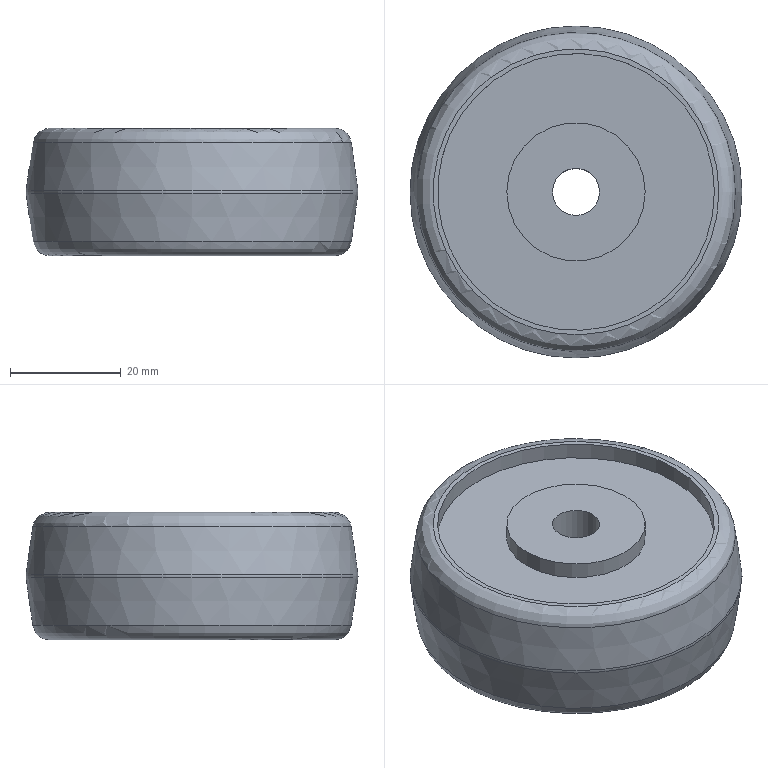Part | STEP file | Transport wheel | 1 solid | 16 faces | box 59.962 x 59.962 x 23 mm | volume 51034 mm3 | plane 6 | cylinder 5 | torus 3 | cone 2 | commonest cylinder face diameters 25 x2 50 x2 8.5 x1
STEP:
#1=CARTESIAN_POINT('',(0.,0.,0.));
#2=DIRECTION('',(0.,0.,1.));
#3=DIRECTION('',(1.,0.,0.));
#4=AXIS2_PLACEMENT_3D('',#1,#2,#3);
#5=CARTESIAN_POINT('',(-29.963,0.,11.772));
#6=VERTEX_POINT('',#5);
#7=CARTESIAN_POINT('',(29.963,0.,11.772));
#8=VERTEX_POINT('',#7);
#9=CARTESIAN_POINT('',(0.,0.,11.772));
#10=DIRECTION('',(0.,0.,1.));
#11=DIRECTION('',(1.,0.,0.));
#12=AXIS2_PLACEMENT_3D('',#9,#10,#11);
#13=CIRCLE('',#12,29.963);
#14=CARTESIAN_POINT('',(0.,0.,11.5));
#15=DIRECTION('',(0.,0.,-1.));
#16=DIRECTION('',(-1.,0.,0.));
#17=AXIS2_PLACEMENT_3D('',#14,#15,#16);
#18=TOROIDAL_SURFACE('',#17,27.981,2.);
#19=CARTESIAN_POINT('',(9.425,6.147));
#20=DIRECTION('',(-1.,0.));
#21=VECTOR('',#20,1.);
#22=LINE('',#19,#21);
#23=(GEOMETRIC_REPRESENTATION_CONTEXT(2)PARAMETRIC_REPRESENTATION_CONTEXT()REPRESENTATION_CONTEXT('',''));
#24=DEFINITIONAL_REPRESENTATION('',(#22),#23);
#25=PCURVE('',#18,#24);
#26=CARTESIAN_POINT('',(0.,0.,23.));
#27=DIRECTION('',(0.,0.,-1.));
#28=DIRECTION('',(-1.,0.,0.));
#29=AXIS2_PLACEMENT_3D('',#26,#27,#28);
#30=CONICAL_SURFACE('',#29,28.419,0.1366);
#31=CARTESIAN_POINT('',(9.425,11.228));
#32=DIRECTION('',(-1.,0.));
#33=VECTOR('',#32,1.);
#34=LINE('',#31,#33);
#35=(GEOMETRIC_REPRESENTATION_CONTEXT(2)PARAMETRIC_REPRESENTATION_CONTEXT()REPRESENTATION_CONTEXT('',''));
#36=DEFINITIONAL_REPRESENTATION('',(#34),#35);
#37=PCURVE('',#30,#36);
#38=SURFACE_CURVE('',#13,(#25,#37),.PCURVE_S1.);
#39=EDGE_CURVE('',#6,#8,#38,.T.);
#40=ORIENTED_EDGE('',*,*,#39,.F.);
#41=CARTESIAN_POINT('',(-29.963,0.,11.228));
#42=VERTEX_POINT('',#41);
#43=CARTESIAN_POINT('',(-29.963,0.,11.772));
#44=CARTESIAN_POINT('',(-29.981,0.,11.637));
#45=CARTESIAN_POINT('',(-29.987,0.,11.5));
#46=CARTESIAN_POINT('',(-29.981,0.,11.363));
#47=CARTESIAN_POINT('',(-29.963,0.,11.228));
#48=B_SPLINE_CURVE_WITH_KNOTS('',4,(#43,#44,#45,#46,#47),.UNSPECIFIED.,.F.,.F.,(5,5),(6.147,6.42),.PIECEWISE_BEZIER_KNOTS.);
#49=CARTESIAN_POINT('',(6.283,0.));
#50=DIRECTION('',(0.,1.));
#51=VECTOR('',#50,1.);
#52=LINE('',#49,#51);
#53=(GEOMETRIC_REPRESENTATION_CONTEXT(2)PARAMETRIC_REPRESENTATION_CONTEXT()REPRESENTATION_CONTEXT('',''));
#54=DEFINITIONAL_REPRESENTATION('',(#52),#53);
#55=PCURVE('',#18,#54);
#56=CARTESIAN_POINT('',(0.,0.));
#57=DIRECTION('',(0.,1.));
#58=VECTOR('',#57,1.);
#59=LINE('',#56,#58);
#60=(GEOMETRIC_REPRESENTATION_CONTEXT(2)PARAMETRIC_REPRESENTATION_CONTEXT()REPRESENTATION_CONTEXT('',''));
#61=DEFINITIONAL_REPRESENTATION('',(#59),#60);
#62=PCURVE('',#18,#61);
#63=SEAM_CURVE('',#48,(#55,#62),.PCURVE_S1.);
#64=EDGE_CURVE('',#6,#42,#63,.T.);
#65=ORIENTED_EDGE('',*,*,#64,.T.);
#66=CARTESIAN_POINT('',(29.963,0.,11.228));
#67=VERTEX_POINT('',#66);
#68=CARTESIAN_POINT('',(0.,0.,11.228));
#69=DIRECTION('',(0.,0.,-1.));
#70=DIRECTION('',(-1.,0.,0.));
#71=AXIS2_PLACEMENT_3D('',#68,#69,#70);
#72=CIRCLE('',#71,29.963);
#73=CARTESIAN_POINT('',(0.,6.42));
#74=DIRECTION('',(1.,0.));
#75=VECTOR('',#74,1.);
#76=LINE('',#73,#75);
#77=(GEOMETRIC_REPRESENTATION_CONTEXT(2)PARAMETRIC_REPRESENTATION_CONTEXT()REPRESENTATION_CONTEXT('',''));
#78=DEFINITIONAL_REPRESENTATION('',(#76),#77);
#79=PCURVE('',#18,#78);
#80=CARTESIAN_POINT('',(0.,0.,11.5));
#81=DIRECTION('',(0.,0.,1.));
#82=DIRECTION('',(1.,0.,0.));
#83=AXIS2_PLACEMENT_3D('',#80,#81,#82);
#84=CONICAL_SURFACE('',#83,30.,0.1366);
#85=CARTESIAN_POINT('',(9.425,-0.2724));
#86=DIRECTION('',(-1.,0.));
#87=VECTOR('',#86,1.);
#88=LINE('',#85,#87);
#89=(GEOMETRIC_REPRESENTATION_CONTEXT(2)PARAMETRIC_REPRESENTATION_CONTEXT()REPRESENTATION_CONTEXT('',''));
#90=DEFINITIONAL_REPRESENTATION('',(#88),#89);
#91=PCURVE('',#84,#90);
#92=SURFACE_CURVE('',#72,(#79,#91),.PCURVE_S1.);
#93=EDGE_CURVE('',#67,#42,#92,.T.);
#94=ORIENTED_EDGE('',*,*,#93,.F.);
#95=CARTESIAN_POINT('',(0.,0.,11.228));
#96=DIRECTION('',(0.,0.,-1.));
#97=DIRECTION('',(-1.,0.,0.));
#98=AXIS2_PLACEMENT_3D('',#95,#96,#97);
#99=CIRCLE('',#98,29.963);
#100=CARTESIAN_POINT('',(0.,6.42));
#101=DIRECTION('',(1.,0.));
#102=VECTOR('',#101,1.);
#103=LINE('',#100,#102);
#104=(GEOMETRIC_REPRESENTATION_CONTEXT(2)PARAMETRIC_REPRESENTATION_CONTEXT()REPRESENTATION_CONTEXT('',''));
#105=DEFINITIONAL_REPRESENTATION('',(#103),#104);
#106=PCURVE('',#18,#105);
#107=CARTESIAN_POINT('',(3.142,-0.2724));
#108=DIRECTION('',(-1.,0.));
#109=VECTOR('',#108,1.);
#110=LINE('',#107,#109);
#111=(GEOMETRIC_REPRESENTATION_CONTEXT(2)PARAMETRIC_REPRESENTATION_CONTEXT()REPRESENTATION_CONTEXT('',''));
#112=DEFINITIONAL_REPRESENTATION('',(#110),#111);
#113=PCURVE('',#84,#112);
#114=SURFACE_CURVE('',#99,(#106,#113),.PCURVE_S1.);
#115=EDGE_CURVE('',#42,#67,#114,.T.);
#116=ORIENTED_EDGE('',*,*,#115,.F.);
#117=ORIENTED_EDGE('',*,*,#64,.F.);
#118=CARTESIAN_POINT('',(0.,0.,11.772));
#119=DIRECTION('',(0.,0.,1.));
#120=DIRECTION('',(1.,0.,0.));
#121=AXIS2_PLACEMENT_3D('',#118,#119,#120);
#122=CIRCLE('',#121,29.963);
#123=CARTESIAN_POINT('',(3.142,6.147));
#124=DIRECTION('',(-1.,0.));
#125=VECTOR('',#124,1.);
#126=LINE('',#123,#125);
#127=(GEOMETRIC_REPRESENTATION_CONTEXT(2)PARAMETRIC_REPRESENTATION_CONTEXT()REPRESENTATION_CONTEXT('',''));
#128=DEFINITIONAL_REPRESENTATION('',(#126),#127);
#129=PCURVE('',#18,#128);
#130=CARTESIAN_POINT('',(9.425,11.228));
#131=DIRECTION('',(-1.,0.));
#132=VECTOR('',#131,1.);
#133=LINE('',#130,#132);
#134=(GEOMETRIC_REPRESENTATION_CONTEXT(2)PARAMETRIC_REPRESENTATION_CONTEXT()REPRESENTATION_CONTEXT('',''));
#135=DEFINITIONAL_REPRESENTATION('',(#133),#134);
#136=PCURVE('',#30,#135);
#137=SURFACE_CURVE('',#122,(#129,#136),.PCURVE_S1.);
#138=EDGE_CURVE('',#8,#6,#137,.T.);
#139=ORIENTED_EDGE('',*,*,#138,.F.);
#140=EDGE_LOOP('',(#40,#65,#94,#116,#117,#139));
#141=FACE_BOUND('',#140,.T.);
#142=ADVANCED_FACE('',(#141),#18,.T.);
#143=CARTESIAN_POINT('',(25.803,0.,23.));
#144=VERTEX_POINT('',#143);
#145=CARTESIAN_POINT('',(0.,0.,23.));
#146=DIRECTION('',(0.,0.,1.));
#147=DIRECTION('',(1.,0.,0.));
#148=AXIS2_PLACEMENT_3D('',#145,#146,#147);
#149=CIRCLE('',#148,25.803);
#150=CARTESIAN_POINT('',(0.,0.,23.));
#151=DIRECTION('',(0.,0.,1.));
#152=DIRECTION('',(1.,0.,0.));
#153=AXIS2_PLACEMENT_3D('',#150,#151,#152);
#154=PLANE('',#153);
#155=CARTESIAN_POINT('',(0.,0.));
#156=DIRECTION('',(1.,0.));
#157=AXIS2_PLACEMENT_2D('',#155,#156);
#158=CIRCLE('',#157,25.803);
#159=(GEOMETRIC_REPRESENTATION_CONTEXT(2)PARAMETRIC_REPRESENTATION_CONTEXT()REPRESENTATION_CONTEXT('',''));
#160=DEFINITIONAL_REPRESENTATION('',(#158),#159);
#161=PCURVE('',#154,#160);
#162=CARTESIAN_POINT('',(0.,0.,20.));
#163=DIRECTION('',(0.,0.,1.));
#164=DIRECTION('',(1.,0.,0.));
#165=AXIS2_PLACEMENT_3D('',#162,#163,#164);
#166=TOROIDAL_SURFACE('',#165,25.803,3.);
#167=CARTESIAN_POINT('',(0.,7.854));
#168=DIRECTION('',(1.,0.));
#169=VECTOR('',#168,1.);
#170=LINE('',#167,#169);
#171=(GEOMETRIC_REPRESENTATION_CONTEXT(2)PARAMETRIC_REPRESENTATION_CONTEXT()REPRESENTATION_CONTEXT('',''));
#172=DEFINITIONAL_REPRESENTATION('',(#170),#171);
#173=PCURVE('',#166,#172);
#174=SURFACE_CURVE('',#149,(#161,#173),.PCURVE_S1.);
#175=EDGE_CURVE('',#144,#144,#174,.T.);
#176=ORIENTED_EDGE('',*,*,#175,.T.);
#177=EDGE_LOOP('',(#176));
#178=FACE_BOUND('',#177,.T.);
#179=CARTESIAN_POINT('',(25.,0.,23.));
#180=VERTEX_POINT('',#179);
#181=CARTESIAN_POINT('',(0.,0.,23.));
#182=DIRECTION('',(0.,0.,1.));
#183=DIRECTION('',(1.,0.,0.));
#184=AXIS2_PLACEMENT_3D('',#181,#182,#183);
#185=CIRCLE('',#184,25.);
#186=CARTESIAN_POINT('',(0.,0.));
#187=DIRECTION('',(1.,0.));
#188=AXIS2_PLACEMENT_2D('',#186,#187);
#189=CIRCLE('',#188,25.);
#190=(GEOMETRIC_REPRESENTATION_CONTEXT(2)PARAMETRIC_REPRESENTATION_CONTEXT()REPRESENTATION_CONTEXT('',''));
#191=DEFINITIONAL_REPRESENTATION('',(#189),#190);
#192=PCURVE('',#154,#191);
#193=CARTESIAN_POINT('',(0.,0.,20.));
#194=DIRECTION('',(0.,0.,1.));
#195=DIRECTION('',(1.,0.,0.));
#196=AXIS2_PLACEMENT_3D('',#193,#194,#195);
#197=CYLINDRICAL_SURFACE('',#196,25.);
#198=CARTESIAN_POINT('',(0.,3.));
#199=DIRECTION('',(1.,0.));
#200=VECTOR('',#199,1.);
#201=LINE('',#198,#200);
#202=(GEOMETRIC_REPRESENTATION_CONTEXT(2)PARAMETRIC_REPRESENTATION_CONTEXT()REPRESENTATION_CONTEXT('',''));
#203=DEFINITIONAL_REPRESENTATION('',(#201),#202);
#204=PCURVE('',#197,#203);
#205=SURFACE_CURVE('',#185,(#192,#204),.PCURVE_S1.);
#206=EDGE_CURVE('',#180,#180,#205,.T.);
#207=ORIENTED_EDGE('',*,*,#206,.F.);
#208=EDGE_LOOP('',(#207));
#209=FACE_BOUND('',#208,.T.);
#210=ADVANCED_FACE('',(#178,#209),#154,.T.);
#211=CARTESIAN_POINT('',(25.803,0.,0.));
#212=VERTEX_POINT('',#211);
#213=CARTESIAN_POINT('',(0.,0.,0.));
#214=DIRECTION('',(0.,0.,-1.));
#215=DIRECTION('',(1.,0.,0.));
#216=AXIS2_PLACEMENT_3D('',#213,#214,#215);
#217=CIRCLE('',#216,25.803);
#218=CARTESIAN_POINT('',(0.,0.,0.));
#219=DIRECTION('',(0.,0.,1.));
#220=DIRECTION('',(1.,0.,0.));
#221=AXIS2_PLACEMENT_3D('',#218,#219,#220);
#222=PLANE('',#221);
#223=CARTESIAN_POINT('',(25.803,0.));
#224=CARTESIAN_POINT('',(25.803,-44.693));
#225=CARTESIAN_POINT('',(-12.902,-22.346));
#226=CARTESIAN_POINT('',(-51.607,0.));
#227=CARTESIAN_POINT('',(-12.902,22.346));
#228=CARTESIAN_POINT('',(25.803,44.693));
#229=CARTESIAN_POINT('',(25.803,0.));
#230=(BOUNDED_CURVE()B_SPLINE_CURVE(2,(#223,#224,#225,#226,#227,#228,#229),.UNSPECIFIED.,.T.,.F.)B_SPLINE_CURVE_WITH_KNOTS((1,2,2,2,2,1),(-2.094,0.,2.094,4.189,6.283,8.378),.UNSPECIFIED.)CURVE()GEOMETRIC_REPRESENTATION_ITEM()RATIONAL_B_SPLINE_CURVE((1.,0.5,1.,0.5,1.,0.5,1.))REPRESENTATION_ITEM(''));
#231=(GEOMETRIC_REPRESENTATION_CONTEXT(2)PARAMETRIC_REPRESENTATION_CONTEXT()REPRESENTATION_CONTEXT('',''));
#232=DEFINITIONAL_REPRESENTATION('',(#230),#231);
#233=PCURVE('',#222,#232);
#234=CARTESIAN_POINT('',(0.,0.,3.));
#235=DIRECTION('',(0.,0.,1.));
#236=DIRECTION('',(1.,0.,0.));
#237=AXIS2_PLACEMENT_3D('',#234,#235,#236);
#238=TOROIDAL_SURFACE('',#237,25.803,3.);
#239=CARTESIAN_POINT('',(6.283,4.712));
#240=DIRECTION('',(-1.,0.));
#241=VECTOR('',#240,1.);
#242=LINE('',#239,#241);
#243=(GEOMETRIC_REPRESENTATION_CONTEXT(2)PARAMETRIC_REPRESENTATION_CONTEXT()REPRESENTATION_CONTEXT('',''));
#244=DEFINITIONAL_REPRESENTATION('',(#242),#243);
#245=PCURVE('',#238,#244);
#246=SURFACE_CURVE('',#217,(#233,#245),.PCURVE_S1.);
#247=EDGE_CURVE('',#212,#212,#246,.T.);
#248=ORIENTED_EDGE('',*,*,#247,.T.);
#249=EDGE_LOOP('',(#248));
#250=FACE_BOUND('',#249,.T.);
#251=CARTESIAN_POINT('',(-25.,0.,0.));
#252=VERTEX_POINT('',#251);
#253=CARTESIAN_POINT('',(0.,0.,0.));
#254=DIRECTION('',(0.,0.,-1.));
#255=DIRECTION('',(-1.,0.,0.));
#256=AXIS2_PLACEMENT_3D('',#253,#254,#255);
#257=CIRCLE('',#256,25.);
#258=CARTESIAN_POINT('',(-25.,0.));
#259=CARTESIAN_POINT('',(-25.,43.301));
#260=CARTESIAN_POINT('',(12.5,21.651));
#261=CARTESIAN_POINT('',(50.,0.));
#262=CARTESIAN_POINT('',(12.5,-21.651));
#263=CARTESIAN_POINT('',(-25.,-43.301));
#264=CARTESIAN_POINT('',(-25.,0.));
#265=(BOUNDED_CURVE()B_SPLINE_CURVE(2,(#258,#259,#260,#261,#262,#263,#264),.UNSPECIFIED.,.T.,.F.)B_SPLINE_CURVE_WITH_KNOTS((1,2,2,2,2,1),(-2.094,0.,2.094,4.189,6.283,8.378),.UNSPECIFIED.)CURVE()GEOMETRIC_REPRESENTATION_ITEM()RATIONAL_B_SPLINE_CURVE((1.,0.5,1.,0.5,1.,0.5,1.))REPRESENTATION_ITEM(''));
#266=(GEOMETRIC_REPRESENTATION_CONTEXT(2)PARAMETRIC_REPRESENTATION_CONTEXT()REPRESENTATION_CONTEXT('',''));
#267=DEFINITIONAL_REPRESENTATION('',(#265),#266);
#268=PCURVE('',#222,#267);
#269=CARTESIAN_POINT('',(0.,0.,3.));
#270=DIRECTION('',(0.,0.,-1.));
#271=DIRECTION('',(-1.,0.,0.));
#272=AXIS2_PLACEMENT_3D('',#269,#270,#271);
#273=CYLINDRICAL_SURFACE('',#272,25.);
#274=CARTESIAN_POINT('',(0.,3.));
#275=DIRECTION('',(1.,0.));
#276=VECTOR('',#275,1.);
#277=LINE('',#274,#276);
#278=(GEOMETRIC_REPRESENTATION_CONTEXT(2)PARAMETRIC_REPRESENTATION_CONTEXT()REPRESENTATION_CONTEXT('',''));
#279=DEFINITIONAL_REPRESENTATION('',(#277),#278);
#280=PCURVE('',#273,#279);
#281=SURFACE_CURVE('',#257,(#268,#280),.PCURVE_S1.);
#282=EDGE_CURVE('',#252,#252,#281,.T.);
#283=ORIENTED_EDGE('',*,*,#282,.F.);
#284=EDGE_LOOP('',(#283));
#285=FACE_BOUND('',#284,.T.);
#286=ADVANCED_FACE('',(#250,#285),#222,.F.);
#287=CARTESIAN_POINT('',(4.25,0.,0.));
#288=VERTEX_POINT('',#287);
#289=CARTESIAN_POINT('',(0.,0.,0.));
#290=DIRECTION('',(0.,0.,1.));
#291=DIRECTION('',(1.,0.,0.));
#292=AXIS2_PLACEMENT_3D('',#289,#290,#291);
#293=CIRCLE('',#292,4.25);
#294=CARTESIAN_POINT('',(0.,0.,0.));
#295=DIRECTION('',(0.,0.,1.));
#296=DIRECTION('',(1.,0.,0.));
#297=AXIS2_PLACEMENT_3D('',#294,#295,#296);
#298=PLANE('',#297);
#299=CARTESIAN_POINT('',(0.,0.));
#300=DIRECTION('',(1.,0.));
#301=AXIS2_PLACEMENT_2D('',#299,#300);
#302=CIRCLE('',#301,4.25);
#303=(GEOMETRIC_REPRESENTATION_CONTEXT(2)PARAMETRIC_REPRESENTATION_CONTEXT()REPRESENTATION_CONTEXT('',''));
#304=DEFINITIONAL_REPRESENTATION('',(#302),#303);
#305=PCURVE('',#298,#304);
#306=CARTESIAN_POINT('',(0.,0.,0.));
#307=DIRECTION('',(0.,0.,1.));
#308=DIRECTION('',(1.,0.,0.));
#309=AXIS2_PLACEMENT_3D('',#306,#307,#308);
#310=CYLINDRICAL_SURFACE('',#309,4.25);
#311=CARTESIAN_POINT('',(0.,0.));
#312=DIRECTION('',(1.,0.));
#313=VECTOR('',#312,1.);
#314=LINE('',#311,#313);
#315=(GEOMETRIC_REPRESENTATION_CONTEXT(2)PARAMETRIC_REPRESENTATION_CONTEXT()REPRESENTATION_CONTEXT('',''));
#316=DEFINITIONAL_REPRESENTATION('',(#314),#315);
#317=PCURVE('',#310,#316);
#318=SURFACE_CURVE('',#293,(#305,#317),.PCURVE_S1.);
#319=EDGE_CURVE('',#288,#288,#318,.T.);
#320=ORIENTED_EDGE('',*,*,#319,.T.);
#321=EDGE_LOOP('',(#320));
#322=FACE_BOUND('',#321,.T.);
#323=CARTESIAN_POINT('',(-12.5,0.,0.));
#324=VERTEX_POINT('',#323);
#325=CARTESIAN_POINT('',(0.,0.,0.));
#326=DIRECTION('',(0.,0.,-1.));
#327=DIRECTION('',(-1.,0.,0.));
#328=AXIS2_PLACEMENT_3D('',#325,#326,#327);
#329=CIRCLE('',#328,12.5);
#330=CARTESIAN_POINT('',(-12.5,0.));
#331=CARTESIAN_POINT('',(-12.5,21.651));
#332=CARTESIAN_POINT('',(6.25,10.825));
#333=CARTESIAN_POINT('',(25.,0.));
#334=CARTESIAN_POINT('',(6.25,-10.825));
#335=CARTESIAN_POINT('',(-12.5,-21.651));
#336=CARTESIAN_POINT('',(-12.5,0.));
#337=(BOUNDED_CURVE()B_SPLINE_CURVE(2,(#330,#331,#332,#333,#334,#335,#336),.UNSPECIFIED.,.T.,.F.)B_SPLINE_CURVE_WITH_KNOTS((1,2,2,2,2,1),(-2.094,0.,2.094,4.189,6.283,8.378),.UNSPECIFIED.)CURVE()GEOMETRIC_REPRESENTATION_ITEM()RATIONAL_B_SPLINE_CURVE((1.,0.5,1.,0.5,1.,0.5,1.))REPRESENTATION_ITEM(''));
#338=(GEOMETRIC_REPRESENTATION_CONTEXT(2)PARAMETRIC_REPRESENTATION_CONTEXT()REPRESENTATION_CONTEXT('',''));
#339=DEFINITIONAL_REPRESENTATION('',(#337),#338);
#340=PCURVE('',#298,#339);
#341=CARTESIAN_POINT('',(0.,0.,3.));
#342=DIRECTION('',(0.,0.,-1.));
#343=DIRECTION('',(-1.,0.,0.));
#344=AXIS2_PLACEMENT_3D('',#341,#342,#343);
#345=CYLINDRICAL_SURFACE('',#344,12.5);
#346=CARTESIAN_POINT('',(0.,3.));
#347=DIRECTION('',(1.,0.));
#348=VECTOR('',#347,1.);
#349=LINE('',#346,#348);
#350=(GEOMETRIC_REPRESENTATION_CONTEXT(2)PARAMETRIC_REPRESENTATION_CONTEXT()REPRESENTATION_CONTEXT('',''));
#351=DEFINITIONAL_REPRESENTATION('',(#349),#350);
#352=PCURVE('',#345,#351);
#353=SURFACE_CURVE('',#329,(#340,#352),.PCURVE_S1.);
#354=EDGE_CURVE('',#324,#324,#353,.T.);
#355=ORIENTED_EDGE('',*,*,#354,.T.);
#356=EDGE_LOOP('',(#355));
#357=FACE_BOUND('',#356,.T.);
#358=ADVANCED_FACE('',(#322,#357),#298,.F.);
#359=CARTESIAN_POINT('',(4.25,0.,23.));
#360=VERTEX_POINT('',#359);
#361=CARTESIAN_POINT('',(0.,0.,23.));
#362=DIRECTION('',(0.,0.,1.));
#363=DIRECTION('',(1.,0.,0.));
#364=AXIS2_PLACEMENT_3D('',#361,#362,#363);
#365=CIRCLE('',#364,4.25);
#366=CARTESIAN_POINT('',(0.,0.,23.));
#367=DIRECTION('',(0.,0.,1.));
#368=DIRECTION('',(1.,0.,0.));
#369=AXIS2_PLACEMENT_3D('',#366,#367,#368);
#370=PLANE('',#369);
#371=CARTESIAN_POINT('',(0.,0.));
#372=DIRECTION('',(1.,0.));
#373=AXIS2_PLACEMENT_2D('',#371,#372);
#374=CIRCLE('',#373,4.25);
#375=(GEOMETRIC_REPRESENTATION_CONTEXT(2)PARAMETRIC_REPRESENTATION_CONTEXT()REPRESENTATION_CONTEXT('',''));
#376=DEFINITIONAL_REPRESENTATION('',(#374),#375);
#377=PCURVE('',#370,#376);
#378=CARTESIAN_POINT('',(0.,23.));
#379=DIRECTION('',(1.,0.));
#380=VECTOR('',#379,1.);
#381=LINE('',#378,#380);
#382=(GEOMETRIC_REPRESENTATION_CONTEXT(2)PARAMETRIC_REPRESENTATION_CONTEXT()REPRESENTATION_CONTEXT('',''));
#383=DEFINITIONAL_REPRESENTATION('',(#381),#382);
#384=PCURVE('',#310,#383);
#385=SURFACE_CURVE('',#365,(#377,#384),.PCURVE_S1.);
#386=EDGE_CURVE('',#360,#360,#385,.T.);
#387=ORIENTED_EDGE('',*,*,#386,.F.);
#388=EDGE_LOOP('',(#387));
#389=FACE_BOUND('',#388,.T.);
#390=CARTESIAN_POINT('',(12.5,0.,23.));
#391=VERTEX_POINT('',#390);
#392=CARTESIAN_POINT('',(0.,0.,23.));
#393=DIRECTION('',(0.,0.,1.));
#394=DIRECTION('',(1.,0.,0.));
#395=AXIS2_PLACEMENT_3D('',#392,#393,#394);
#396=CIRCLE('',#395,12.5);
#397=CARTESIAN_POINT('',(0.,0.));
#398=DIRECTION('',(1.,0.));
#399=AXIS2_PLACEMENT_2D('',#397,#398);
#400=CIRCLE('',#399,12.5);
#401=(GEOMETRIC_REPRESENTATION_CONTEXT(2)PARAMETRIC_REPRESENTATION_CONTEXT()REPRESENTATION_CONTEXT('',''));
#402=DEFINITIONAL_REPRESENTATION('',(#400),#401);
#403=PCURVE('',#370,#402);
#404=CARTESIAN_POINT('',(0.,0.,20.));
#405=DIRECTION('',(0.,0.,1.));
#406=DIRECTION('',(1.,0.,0.));
#407=AXIS2_PLACEMENT_3D('',#404,#405,#406);
#408=CYLINDRICAL_SURFACE('',#407,12.5);
#409=CARTESIAN_POINT('',(0.,3.));
#410=DIRECTION('',(1.,0.));
#411=VECTOR('',#410,1.);
#412=LINE('',#409,#411);
#413=(GEOMETRIC_REPRESENTATION_CONTEXT(2)PARAMETRIC_REPRESENTATION_CONTEXT()REPRESENTATION_CONTEXT('',''));
#414=DEFINITIONAL_REPRESENTATION('',(#412),#413);
#415=PCURVE('',#408,#414);
#416=SURFACE_CURVE('',#396,(#403,#415),.PCURVE_S1.);
#417=EDGE_CURVE('',#391,#391,#416,.T.);
#418=ORIENTED_EDGE('',*,*,#417,.T.);
#419=EDGE_LOOP('',(#418));
#420=FACE_BOUND('',#419,.T.);
#421=ADVANCED_FACE('',(#389,#420),#370,.T.);
#422=ORIENTED_EDGE('',*,*,#319,.T.);
#423=CARTESIAN_POINT('',(4.25,0.,0.));
#424=CARTESIAN_POINT('',(4.25,0.,23.));
#425=B_SPLINE_CURVE_WITH_KNOTS('',1,(#423,#424),.UNSPECIFIED.,.F.,.F.,(2,2),(0.,23.),.PIECEWISE_BEZIER_KNOTS.);
#426=CARTESIAN_POINT('',(6.283,0.));
#427=DIRECTION('',(0.,1.));
#428=VECTOR('',#427,1.);
#429=LINE('',#426,#428);
#430=(GEOMETRIC_REPRESENTATION_CONTEXT(2)PARAMETRIC_REPRESENTATION_CONTEXT()REPRESENTATION_CONTEXT('',''));
#431=DEFINITIONAL_REPRESENTATION('',(#429),#430);
#432=PCURVE('',#310,#431);
#433=CARTESIAN_POINT('',(0.,0.));
#434=DIRECTION('',(0.,1.));
#435=VECTOR('',#434,1.);
#436=LINE('',#433,#435);
#437=(GEOMETRIC_REPRESENTATION_CONTEXT(2)PARAMETRIC_REPRESENTATION_CONTEXT()REPRESENTATION_CONTEXT('',''));
#438=DEFINITIONAL_REPRESENTATION('',(#436),#437);
#439=PCURVE('',#310,#438);
#440=SEAM_CURVE('',#425,(#432,#439),.PCURVE_S1.);
#441=EDGE_CURVE('',#288,#360,#440,.T.);
#442=ORIENTED_EDGE('',*,*,#441,.T.);
#443=ORIENTED_EDGE('',*,*,#386,.F.);
#444=ORIENTED_EDGE('',*,*,#441,.F.);
#445=EDGE_LOOP('',(#422,#442,#443,#444));
#446=FACE_BOUND('',#445,.F.);
#447=ADVANCED_FACE('',(#446),#310,.F.);
#448=CARTESIAN_POINT('',(25.,0.,20.));
#449=VERTEX_POINT('',#448);
#450=CARTESIAN_POINT('',(0.,0.,20.));
#451=DIRECTION('',(0.,0.,1.));
#452=DIRECTION('',(1.,0.,0.));
#453=AXIS2_PLACEMENT_3D('',#450,#451,#452);
#454=CIRCLE('',#453,25.);
#455=CARTESIAN_POINT('',(0.,0.));
#456=DIRECTION('',(1.,0.));
#457=VECTOR('',#456,1.);
#458=LINE('',#455,#457);
#459=(GEOMETRIC_REPRESENTATION_CONTEXT(2)PARAMETRIC_REPRESENTATION_CONTEXT()REPRESENTATION_CONTEXT('',''));
#460=DEFINITIONAL_REPRESENTATION('',(#458),#459);
#461=PCURVE('',#197,#460);
#462=CARTESIAN_POINT('',(0.,0.,20.));
#463=DIRECTION('',(0.,0.,1.));
#464=DIRECTION('',(1.,0.,0.));
#465=AXIS2_PLACEMENT_3D('',#462,#463,#464);
#466=PLANE('',#465);
#467=CARTESIAN_POINT('',(0.,0.));
#468=DIRECTION('',(1.,0.));
#469=AXIS2_PLACEMENT_2D('',#467,#468);
#470=CIRCLE('',#469,25.);
#471=(GEOMETRIC_REPRESENTATION_CONTEXT(2)PARAMETRIC_REPRESENTATION_CONTEXT()REPRESENTATION_CONTEXT('',''));
#472=DEFINITIONAL_REPRESENTATION('',(#470),#471);
#473=PCURVE('',#466,#472);
#474=SURFACE_CURVE('',#454,(#461,#473),.PCURVE_S1.);
#475=EDGE_CURVE('',#449,#449,#474,.T.);
#476=ORIENTED_EDGE('',*,*,#475,.T.);
#477=CARTESIAN_POINT('',(25.,0.,20.));
#478=CARTESIAN_POINT('',(25.,0.,23.));
#479=B_SPLINE_CURVE_WITH_KNOTS('',1,(#477,#478),.UNSPECIFIED.,.F.,.F.,(2,2),(0.,3.),.PIECEWISE_BEZIER_KNOTS.);
#480=CARTESIAN_POINT('',(6.283,0.));
#481=DIRECTION('',(0.,1.));
#482=VECTOR('',#481,1.);
#483=LINE('',#480,#482);
#484=(GEOMETRIC_REPRESENTATION_CONTEXT(2)PARAMETRIC_REPRESENTATION_CONTEXT()REPRESENTATION_CONTEXT('',''));
#485=DEFINITIONAL_REPRESENTATION('',(#483),#484);
#486=PCURVE('',#197,#485);
#487=CARTESIAN_POINT('',(0.,0.));
#488=DIRECTION('',(0.,1.));
#489=VECTOR('',#488,1.);
#490=LINE('',#487,#489);
#491=(GEOMETRIC_REPRESENTATION_CONTEXT(2)PARAMETRIC_REPRESENTATION_CONTEXT()REPRESENTATION_CONTEXT('',''));
#492=DEFINITIONAL_REPRESENTATION('',(#490),#491);
#493=PCURVE('',#197,#492);
#494=SEAM_CURVE('',#479,(#486,#493),.PCURVE_S1.);
#495=EDGE_CURVE('',#449,#180,#494,.T.);
#496=ORIENTED_EDGE('',*,*,#495,.T.);
#497=ORIENTED_EDGE('',*,*,#206,.F.);
#498=ORIENTED_EDGE('',*,*,#495,.F.);
#499=EDGE_LOOP('',(#476,#496,#497,#498));
#500=FACE_BOUND('',#499,.F.);
#501=ADVANCED_FACE('',(#500),#197,.F.);
#502=CARTESIAN_POINT('',(12.5,0.,20.));
#503=VERTEX_POINT('',#502);
#504=CARTESIAN_POINT('',(0.,0.,20.));
#505=DIRECTION('',(0.,0.,1.));
#506=DIRECTION('',(1.,0.,0.));
#507=AXIS2_PLACEMENT_3D('',#504,#505,#506);
#508=CIRCLE('',#507,12.5);
#509=CARTESIAN_POINT('',(0.,0.));
#510=DIRECTION('',(1.,0.));
#511=AXIS2_PLACEMENT_2D('',#509,#510);
#512=CIRCLE('',#511,12.5);
#513=(GEOMETRIC_REPRESENTATION_CONTEXT(2)PARAMETRIC_REPRESENTATION_CONTEXT()REPRESENTATION_CONTEXT('',''));
#514=DEFINITIONAL_REPRESENTATION('',(#512),#513);
#515=PCURVE('',#466,#514);
#516=CARTESIAN_POINT('',(0.,0.));
#517=DIRECTION('',(1.,0.));
#518=VECTOR('',#517,1.);
#519=LINE('',#516,#518);
#520=(GEOMETRIC_REPRESENTATION_CONTEXT(2)PARAMETRIC_REPRESENTATION_CONTEXT()REPRESENTATION_CONTEXT('',''));
#521=DEFINITIONAL_REPRESENTATION('',(#519),#520);
#522=PCURVE('',#408,#521);
#523=SURFACE_CURVE('',#508,(#515,#522),.PCURVE_S1.);
#524=EDGE_CURVE('',#503,#503,#523,.T.);
#525=ORIENTED_EDGE('',*,*,#524,.F.);
#526=EDGE_LOOP('',(#525));
#527=FACE_BOUND('',#526,.T.);
#528=ORIENTED_EDGE('',*,*,#475,.T.);
#529=EDGE_LOOP('',(#528));
#530=FACE_BOUND('',#529,.T.);
#531=ADVANCED_FACE('',(#527,#530),#466,.T.);
#532=ORIENTED_EDGE('',*,*,#524,.T.);
#533=CARTESIAN_POINT('',(12.5,0.,20.));
#534=CARTESIAN_POINT('',(12.5,0.,23.));
#535=B_SPLINE_CURVE_WITH_KNOTS('',1,(#533,#534),.UNSPECIFIED.,.F.,.F.,(2,2),(0.,3.),.PIECEWISE_BEZIER_KNOTS.);
#536=CARTESIAN_POINT('',(6.283,0.));
#537=DIRECTION('',(0.,1.));
#538=VECTOR('',#537,1.);
#539=LINE('',#536,#538);
#540=(GEOMETRIC_REPRESENTATION_CONTEXT(2)PARAMETRIC_REPRESENTATION_CONTEXT()REPRESENTATION_CONTEXT('',''));
#541=DEFINITIONAL_REPRESENTATION('',(#539),#540);
#542=PCURVE('',#408,#541);
#543=CARTESIAN_POINT('',(0.,0.));
#544=DIRECTION('',(0.,1.));
#545=VECTOR('',#544,1.);
#546=LINE('',#543,#545);
#547=(GEOMETRIC_REPRESENTATION_CONTEXT(2)PARAMETRIC_REPRESENTATION_CONTEXT()REPRESENTATION_CONTEXT('',''));
#548=DEFINITIONAL_REPRESENTATION('',(#546),#547);
#549=PCURVE('',#408,#548);
#550=SEAM_CURVE('',#535,(#542,#549),.PCURVE_S1.);
#551=EDGE_CURVE('',#503,#391,#550,.T.);
#552=ORIENTED_EDGE('',*,*,#551,.T.);
#553=ORIENTED_EDGE('',*,*,#417,.F.);
#554=ORIENTED_EDGE('',*,*,#551,.F.);
#555=EDGE_LOOP('',(#532,#552,#553,#554));
#556=FACE_BOUND('',#555,.T.);
#557=ADVANCED_FACE('',(#556),#408,.T.);
#558=CARTESIAN_POINT('',(-25.,0.,3.));
#559=VERTEX_POINT('',#558);
#560=CARTESIAN_POINT('',(0.,0.,3.));
#561=DIRECTION('',(0.,0.,-1.));
#562=DIRECTION('',(-1.,0.,0.));
#563=AXIS2_PLACEMENT_3D('',#560,#561,#562);
#564=CIRCLE('',#563,25.);
#565=CARTESIAN_POINT('',(0.,0.));
#566=DIRECTION('',(1.,0.));
#567=VECTOR('',#566,1.);
#568=LINE('',#565,#567);
#569=(GEOMETRIC_REPRESENTATION_CONTEXT(2)PARAMETRIC_REPRESENTATION_CONTEXT()REPRESENTATION_CONTEXT('',''));
#570=DEFINITIONAL_REPRESENTATION('',(#568),#569);
#571=PCURVE('',#273,#570);
#572=CARTESIAN_POINT('',(0.,0.,3.));
#573=DIRECTION('',(0.,0.,-1.));
#574=DIRECTION('',(-1.,0.,0.));
#575=AXIS2_PLACEMENT_3D('',#572,#573,#574);
#576=PLANE('',#575);
#577=CARTESIAN_POINT('',(0.,0.));
#578=DIRECTION('',(1.,0.));
#579=AXIS2_PLACEMENT_2D('',#577,#578);
#580=CIRCLE('',#579,25.);
#581=(GEOMETRIC_REPRESENTATION_CONTEXT(2)PARAMETRIC_REPRESENTATION_CONTEXT()REPRESENTATION_CONTEXT('',''));
#582=DEFINITIONAL_REPRESENTATION('',(#580),#581);
#583=PCURVE('',#576,#582);
#584=SURFACE_CURVE('',#564,(#571,#583),.PCURVE_S1.);
#585=EDGE_CURVE('',#559,#559,#584,.T.);
#586=ORIENTED_EDGE('',*,*,#585,.T.);
#587=CARTESIAN_POINT('',(-25.,0.,3.));
#588=CARTESIAN_POINT('',(-25.,0.,0.));
#589=B_SPLINE_CURVE_WITH_KNOTS('',1,(#587,#588),.UNSPECIFIED.,.F.,.F.,(2,2),(0.,3.),.PIECEWISE_BEZIER_KNOTS.);
#590=CARTESIAN_POINT('',(6.283,0.));
#591=DIRECTION('',(0.,1.));
#592=VECTOR('',#591,1.);
#593=LINE('',#590,#592);
#594=(GEOMETRIC_REPRESENTATION_CONTEXT(2)PARAMETRIC_REPRESENTATION_CONTEXT()REPRESENTATION_CONTEXT('',''));
#595=DEFINITIONAL_REPRESENTATION('',(#593),#594);
#596=PCURVE('',#273,#595);
#597=CARTESIAN_POINT('',(0.,0.));
#598=DIRECTION('',(0.,1.));
#599=VECTOR('',#598,1.);
#600=LINE('',#597,#599);
#601=(GEOMETRIC_REPRESENTATION_CONTEXT(2)PARAMETRIC_REPRESENTATION_CONTEXT()REPRESENTATION_CONTEXT('',''));
#602=DEFINITIONAL_REPRESENTATION('',(#600),#601);
#603=PCURVE('',#273,#602);
#604=SEAM_CURVE('',#589,(#596,#603),.PCURVE_S1.);
#605=EDGE_CURVE('',#559,#252,#604,.T.);
#606=ORIENTED_EDGE('',*,*,#605,.T.);
#607=ORIENTED_EDGE('',*,*,#282,.F.);
#608=ORIENTED_EDGE('',*,*,#605,.F.);
#609=EDGE_LOOP('',(#586,#606,#607,#608));
#610=FACE_BOUND('',#609,.F.);
#611=ADVANCED_FACE('',(#610),#273,.F.);
#612=CARTESIAN_POINT('',(-12.5,0.,3.));
#613=VERTEX_POINT('',#612);
#614=CARTESIAN_POINT('',(0.,0.,3.));
#615=DIRECTION('',(0.,0.,-1.));
#616=DIRECTION('',(-1.,0.,0.));
#617=AXIS2_PLACEMENT_3D('',#614,#615,#616);
#618=CIRCLE('',#617,12.5);
#619=CARTESIAN_POINT('',(0.,0.));
#620=DIRECTION('',(1.,0.));
#621=AXIS2_PLACEMENT_2D('',#619,#620);
#622=CIRCLE('',#621,12.5);
#623=(GEOMETRIC_REPRESENTATION_CONTEXT(2)PARAMETRIC_REPRESENTATION_CONTEXT()REPRESENTATION_CONTEXT('',''));
#624=DEFINITIONAL_REPRESENTATION('',(#622),#623);
#625=PCURVE('',#576,#624);
#626=CARTESIAN_POINT('',(0.,0.));
#627=DIRECTION('',(1.,0.));
#628=VECTOR('',#627,1.);
#629=LINE('',#626,#628);
#630=(GEOMETRIC_REPRESENTATION_CONTEXT(2)PARAMETRIC_REPRESENTATION_CONTEXT()REPRESENTATION_CONTEXT('',''));
#631=DEFINITIONAL_REPRESENTATION('',(#629),#630);
#632=PCURVE('',#345,#631);
#633=SURFACE_CURVE('',#618,(#625,#632),.PCURVE_S1.);
#634=EDGE_CURVE('',#613,#613,#633,.T.);
#635=ORIENTED_EDGE('',*,*,#634,.F.);
#636=EDGE_LOOP('',(#635));
#637=FACE_BOUND('',#636,.T.);
#638=ORIENTED_EDGE('',*,*,#585,.T.);
#639=EDGE_LOOP('',(#638));
#640=FACE_BOUND('',#639,.T.);
#641=ADVANCED_FACE('',(#637,#640),#576,.T.);
#642=ORIENTED_EDGE('',*,*,#634,.T.);
#643=CARTESIAN_POINT('',(-12.5,0.,3.));
#644=CARTESIAN_POINT('',(-12.5,0.,0.));
#645=B_SPLINE_CURVE_WITH_KNOTS('',1,(#643,#644),.UNSPECIFIED.,.F.,.F.,(2,2),(0.,3.),.PIECEWISE_BEZIER_KNOTS.);
#646=CARTESIAN_POINT('',(6.283,0.));
#647=DIRECTION('',(0.,1.));
#648=VECTOR('',#647,1.);
#649=LINE('',#646,#648);
#650=(GEOMETRIC_REPRESENTATION_CONTEXT(2)PARAMETRIC_REPRESENTATION_CONTEXT()REPRESENTATION_CONTEXT('',''));
#651=DEFINITIONAL_REPRESENTATION('',(#649),#650);
#652=PCURVE('',#345,#651);
#653=CARTESIAN_POINT('',(0.,0.));
#654=DIRECTION('',(0.,1.));
#655=VECTOR('',#654,1.);
#656=LINE('',#653,#655);
#657=(GEOMETRIC_REPRESENTATION_CONTEXT(2)PARAMETRIC_REPRESENTATION_CONTEXT()REPRESENTATION_CONTEXT('',''));
#658=DEFINITIONAL_REPRESENTATION('',(#656),#657);
#659=PCURVE('',#345,#658);
#660=SEAM_CURVE('',#645,(#652,#659),.PCURVE_S1.);
#661=EDGE_CURVE('',#613,#324,#660,.T.);
#662=ORIENTED_EDGE('',*,*,#661,.T.);
#663=ORIENTED_EDGE('',*,*,#354,.F.);
#664=ORIENTED_EDGE('',*,*,#661,.F.);
#665=EDGE_LOOP('',(#642,#662,#663,#664));
#666=FACE_BOUND('',#665,.T.);
#667=ADVANCED_FACE('',(#666),#345,.T.);
#668=CARTESIAN_POINT('',(28.775,0.,20.409));
#669=VERTEX_POINT('',#668);
#670=CARTESIAN_POINT('',(0.,0.,20.409));
#671=DIRECTION('',(0.,0.,-1.));
#672=DIRECTION('',(1.,0.,0.));
#673=AXIS2_PLACEMENT_3D('',#670,#671,#672);
#674=CIRCLE('',#673,28.775);
#675=CARTESIAN_POINT('',(3.142,2.591));
#676=DIRECTION('',(1.,0.));
#677=VECTOR('',#676,1.);
#678=LINE('',#675,#677);
#679=(GEOMETRIC_REPRESENTATION_CONTEXT(2)PARAMETRIC_REPRESENTATION_CONTEXT()REPRESENTATION_CONTEXT('',''));
#680=DEFINITIONAL_REPRESENTATION('',(#678),#679);
#681=PCURVE('',#30,#680);
#682=CARTESIAN_POINT('',(6.283,6.42));
#683=DIRECTION('',(-1.,0.));
#684=VECTOR('',#683,1.);
#685=LINE('',#682,#684);
#686=(GEOMETRIC_REPRESENTATION_CONTEXT(2)PARAMETRIC_REPRESENTATION_CONTEXT()REPRESENTATION_CONTEXT('',''));
#687=DEFINITIONAL_REPRESENTATION('',(#685),#686);
#688=PCURVE('',#166,#687);
#689=SURFACE_CURVE('',#674,(#681,#688),.PCURVE_S1.);
#690=EDGE_CURVE('',#669,#669,#689,.T.);
#691=ORIENTED_EDGE('',*,*,#690,.T.);
#692=CARTESIAN_POINT('',(28.775,0.,20.409));
#693=CARTESIAN_POINT('',(29.963,0.,11.772));
#694=B_SPLINE_CURVE_WITH_KNOTS('',1,(#692,#693),.UNSPECIFIED.,.F.,.F.,(2,2),(2.616,11.333),.PIECEWISE_BEZIER_KNOTS.);
#695=CARTESIAN_POINT('',(9.425,0.));
#696=DIRECTION('',(0.,1.));
#697=VECTOR('',#696,1.);
#698=LINE('',#695,#697);
#699=(GEOMETRIC_REPRESENTATION_CONTEXT(2)PARAMETRIC_REPRESENTATION_CONTEXT()REPRESENTATION_CONTEXT('',''));
#700=DEFINITIONAL_REPRESENTATION('',(#698),#699);
#701=PCURVE('',#30,#700);
#702=CARTESIAN_POINT('',(3.142,0.));
#703=DIRECTION('',(0.,1.));
#704=VECTOR('',#703,1.);
#705=LINE('',#702,#704);
#706=(GEOMETRIC_REPRESENTATION_CONTEXT(2)PARAMETRIC_REPRESENTATION_CONTEXT()REPRESENTATION_CONTEXT('',''));
#707=DEFINITIONAL_REPRESENTATION('',(#705),#706);
#708=PCURVE('',#30,#707);
#709=SEAM_CURVE('',#694,(#701,#708),.PCURVE_S1.);
#710=EDGE_CURVE('',#669,#8,#709,.T.);
#711=ORIENTED_EDGE('',*,*,#710,.T.);
#712=ORIENTED_EDGE('',*,*,#138,.T.);
#713=ORIENTED_EDGE('',*,*,#39,.T.);
#714=ORIENTED_EDGE('',*,*,#710,.F.);
#715=EDGE_LOOP('',(#691,#711,#712,#713,#714));
#716=FACE_BOUND('',#715,.T.);
#717=ADVANCED_FACE('',(#716),#30,.T.);
#718=CARTESIAN_POINT('',(28.775,0.,2.591));
#719=VERTEX_POINT('',#718);
#720=CARTESIAN_POINT('',(0.,0.,2.591));
#721=DIRECTION('',(0.,0.,1.));
#722=DIRECTION('',(1.,0.,0.));
#723=AXIS2_PLACEMENT_3D('',#720,#721,#722);
#724=CIRCLE('',#723,28.775);
#725=CARTESIAN_POINT('',(0.,-8.909));
#726=DIRECTION('',(1.,0.));
#727=VECTOR('',#726,1.);
#728=LINE('',#725,#727);
#729=(GEOMETRIC_REPRESENTATION_CONTEXT(2)PARAMETRIC_REPRESENTATION_CONTEXT()REPRESENTATION_CONTEXT('',''));
#730=DEFINITIONAL_REPRESENTATION('',(#728),#729);
#731=PCURVE('',#84,#730);
#732=CARTESIAN_POINT('',(0.,6.147));
#733=DIRECTION('',(1.,0.));
#734=VECTOR('',#733,1.);
#735=LINE('',#732,#734);
#736=(GEOMETRIC_REPRESENTATION_CONTEXT(2)PARAMETRIC_REPRESENTATION_CONTEXT()REPRESENTATION_CONTEXT('',''));
#737=DEFINITIONAL_REPRESENTATION('',(#735),#736);
#738=PCURVE('',#238,#737);
#739=SURFACE_CURVE('',#724,(#731,#738),.PCURVE_S1.);
#740=EDGE_CURVE('',#719,#719,#739,.T.);
#741=ORIENTED_EDGE('',*,*,#740,.T.);
#742=CARTESIAN_POINT('',(28.775,0.,2.591));
#743=CARTESIAN_POINT('',(29.963,0.,11.228));
#744=B_SPLINE_CURVE_WITH_KNOTS('',1,(#742,#743),.UNSPECIFIED.,.F.,.F.,(2,2),(-8.992,-0.2749),.PIECEWISE_BEZIER_KNOTS.);
#745=CARTESIAN_POINT('',(6.283,0.));
#746=DIRECTION('',(0.,1.));
#747=VECTOR('',#746,1.);
#748=LINE('',#745,#747);
#749=(GEOMETRIC_REPRESENTATION_CONTEXT(2)PARAMETRIC_REPRESENTATION_CONTEXT()REPRESENTATION_CONTEXT('',''));
#750=DEFINITIONAL_REPRESENTATION('',(#748),#749);
#751=PCURVE('',#84,#750);
#752=CARTESIAN_POINT('',(0.,0.));
#753=DIRECTION('',(0.,1.));
#754=VECTOR('',#753,1.);
#755=LINE('',#752,#754);
#756=(GEOMETRIC_REPRESENTATION_CONTEXT(2)PARAMETRIC_REPRESENTATION_CONTEXT()REPRESENTATION_CONTEXT('',''));
#757=DEFINITIONAL_REPRESENTATION('',(#755),#756);
#758=PCURVE('',#84,#757);
#759=SEAM_CURVE('',#744,(#751,#758),.PCURVE_S1.);
#760=EDGE_CURVE('',#719,#67,#759,.T.);
#761=ORIENTED_EDGE('',*,*,#760,.T.);
#762=ORIENTED_EDGE('',*,*,#93,.T.);
#763=ORIENTED_EDGE('',*,*,#115,.T.);
#764=ORIENTED_EDGE('',*,*,#760,.F.);
#765=EDGE_LOOP('',(#741,#761,#762,#763,#764));
#766=FACE_BOUND('',#765,.T.);
#767=ADVANCED_FACE('',(#766),#84,.T.);
#768=ORIENTED_EDGE('',*,*,#247,.F.);
#769=CARTESIAN_POINT('',(25.803,0.,0.));
#770=CARTESIAN_POINT('',(26.533,0.,0.));
#771=CARTESIAN_POINT('',(27.247,0.,0.2114));
#772=CARTESIAN_POINT('',(27.879,0.,0.6199));
#773=CARTESIAN_POINT('',(28.369,0.,1.19));
#774=CARTESIAN_POINT('',(28.676,0.,1.869));
#775=CARTESIAN_POINT('',(28.775,0.,2.591));
#776=(BOUNDED_CURVE()B_SPLINE_CURVE(6,(#769,#770,#771,#772,#773,#774,#775),.UNSPECIFIED.,.F.,.F.)B_SPLINE_CURVE_WITH_KNOTS((7,7),(4.712,6.147),.PIECEWISE_BEZIER_KNOTS.)CURVE()GEOMETRIC_REPRESENTATION_ITEM()RATIONAL_B_SPLINE_CURVE((1.026,1.008,0.9983,0.9949,0.9983,1.008,1.026))REPRESENTATION_ITEM(''));
#777=CARTESIAN_POINT('',(6.283,0.));
#778=DIRECTION('',(0.,1.));
#779=VECTOR('',#778,1.);
#780=LINE('',#777,#779);
#781=(GEOMETRIC_REPRESENTATION_CONTEXT(2)PARAMETRIC_REPRESENTATION_CONTEXT()REPRESENTATION_CONTEXT('',''));
#782=DEFINITIONAL_REPRESENTATION('',(#780),#781);
#783=PCURVE('',#238,#782);
#784=CARTESIAN_POINT('',(0.,0.));
#785=DIRECTION('',(0.,1.));
#786=VECTOR('',#785,1.);
#787=LINE('',#784,#786);
#788=(GEOMETRIC_REPRESENTATION_CONTEXT(2)PARAMETRIC_REPRESENTATION_CONTEXT()REPRESENTATION_CONTEXT('',''));
#789=DEFINITIONAL_REPRESENTATION('',(#787),#788);
#790=PCURVE('',#238,#789);
#791=SEAM_CURVE('',#776,(#783,#790),.PCURVE_S1.);
#792=EDGE_CURVE('',#212,#719,#791,.T.);
#793=ORIENTED_EDGE('',*,*,#792,.T.);
#794=ORIENTED_EDGE('',*,*,#740,.F.);
#795=ORIENTED_EDGE('',*,*,#792,.F.);
#796=EDGE_LOOP('',(#768,#793,#794,#795));
#797=FACE_BOUND('',#796,.T.);
#798=ADVANCED_FACE('',(#797),#238,.T.);
#799=ORIENTED_EDGE('',*,*,#690,.F.);
#800=CARTESIAN_POINT('',(28.775,0.,20.409));
#801=CARTESIAN_POINT('',(28.676,0.,21.131));
#802=CARTESIAN_POINT('',(28.369,0.,21.81));
#803=CARTESIAN_POINT('',(27.879,0.,22.38));
#804=CARTESIAN_POINT('',(27.247,0.,22.789));
#805=CARTESIAN_POINT('',(26.533,0.,23.));
#806=CARTESIAN_POINT('',(25.803,0.,23.));
#807=(BOUNDED_CURVE()B_SPLINE_CURVE(6,(#800,#801,#802,#803,#804,#805,#806),.UNSPECIFIED.,.F.,.F.)B_SPLINE_CURVE_WITH_KNOTS((7,7),(0.1366,1.571),.PIECEWISE_BEZIER_KNOTS.)CURVE()GEOMETRIC_REPRESENTATION_ITEM()RATIONAL_B_SPLINE_CURVE((1.026,1.008,0.9983,0.9949,0.9983,1.008,1.026))REPRESENTATION_ITEM(''));
#808=CARTESIAN_POINT('',(6.283,6.283));
#809=DIRECTION('',(0.,1.));
#810=VECTOR('',#809,1.);
#811=LINE('',#808,#810);
#812=(GEOMETRIC_REPRESENTATION_CONTEXT(2)PARAMETRIC_REPRESENTATION_CONTEXT()REPRESENTATION_CONTEXT('',''));
#813=DEFINITIONAL_REPRESENTATION('',(#811),#812);
#814=PCURVE('',#166,#813);
#815=CARTESIAN_POINT('',(0.,6.283));
#816=DIRECTION('',(0.,1.));
#817=VECTOR('',#816,1.);
#818=LINE('',#815,#817);
#819=(GEOMETRIC_REPRESENTATION_CONTEXT(2)PARAMETRIC_REPRESENTATION_CONTEXT()REPRESENTATION_CONTEXT('',''));
#820=DEFINITIONAL_REPRESENTATION('',(#818),#819);
#821=PCURVE('',#166,#820);
#822=SEAM_CURVE('',#807,(#814,#821),.PCURVE_S1.);
#823=EDGE_CURVE('',#669,#144,#822,.T.);
#824=ORIENTED_EDGE('',*,*,#823,.T.);
#825=ORIENTED_EDGE('',*,*,#175,.F.);
#826=ORIENTED_EDGE('',*,*,#823,.F.);
#827=EDGE_LOOP('',(#799,#824,#825,#826));
#828=FACE_BOUND('',#827,.T.);
#829=ADVANCED_FACE('',(#828),#166,.T.);
#830=CLOSED_SHELL('',(#142,#210,#286,#358,#421,#447,#501,#531,#557,#611,#641,#667,#717,#767,#798,#829));
#831=MANIFOLD_SOLID_BREP('',#830);
#832=(LENGTH_UNIT()NAMED_UNIT(*)SI_UNIT(.MILLI.,.METRE.));
#833=UNCERTAINTY_MEASURE_WITH_UNIT(LENGTH_MEASURE(0.00001),#832,'','');
#834=(NAMED_UNIT(*)PLANE_ANGLE_UNIT()SI_UNIT($,.RADIAN.));
#835=(NAMED_UNIT(*)SI_UNIT($,.STERADIAN.)SOLID_ANGLE_UNIT());
#836=(GEOMETRIC_REPRESENTATION_CONTEXT(3)GLOBAL_UNCERTAINTY_ASSIGNED_CONTEXT((#833))GLOBAL_UNIT_ASSIGNED_CONTEXT((#832,#834,#835))REPRESENTATION_CONTEXT('',''));
#837=ADVANCED_BREP_SHAPE_REPRESENTATION('',(#4,#831),#836);